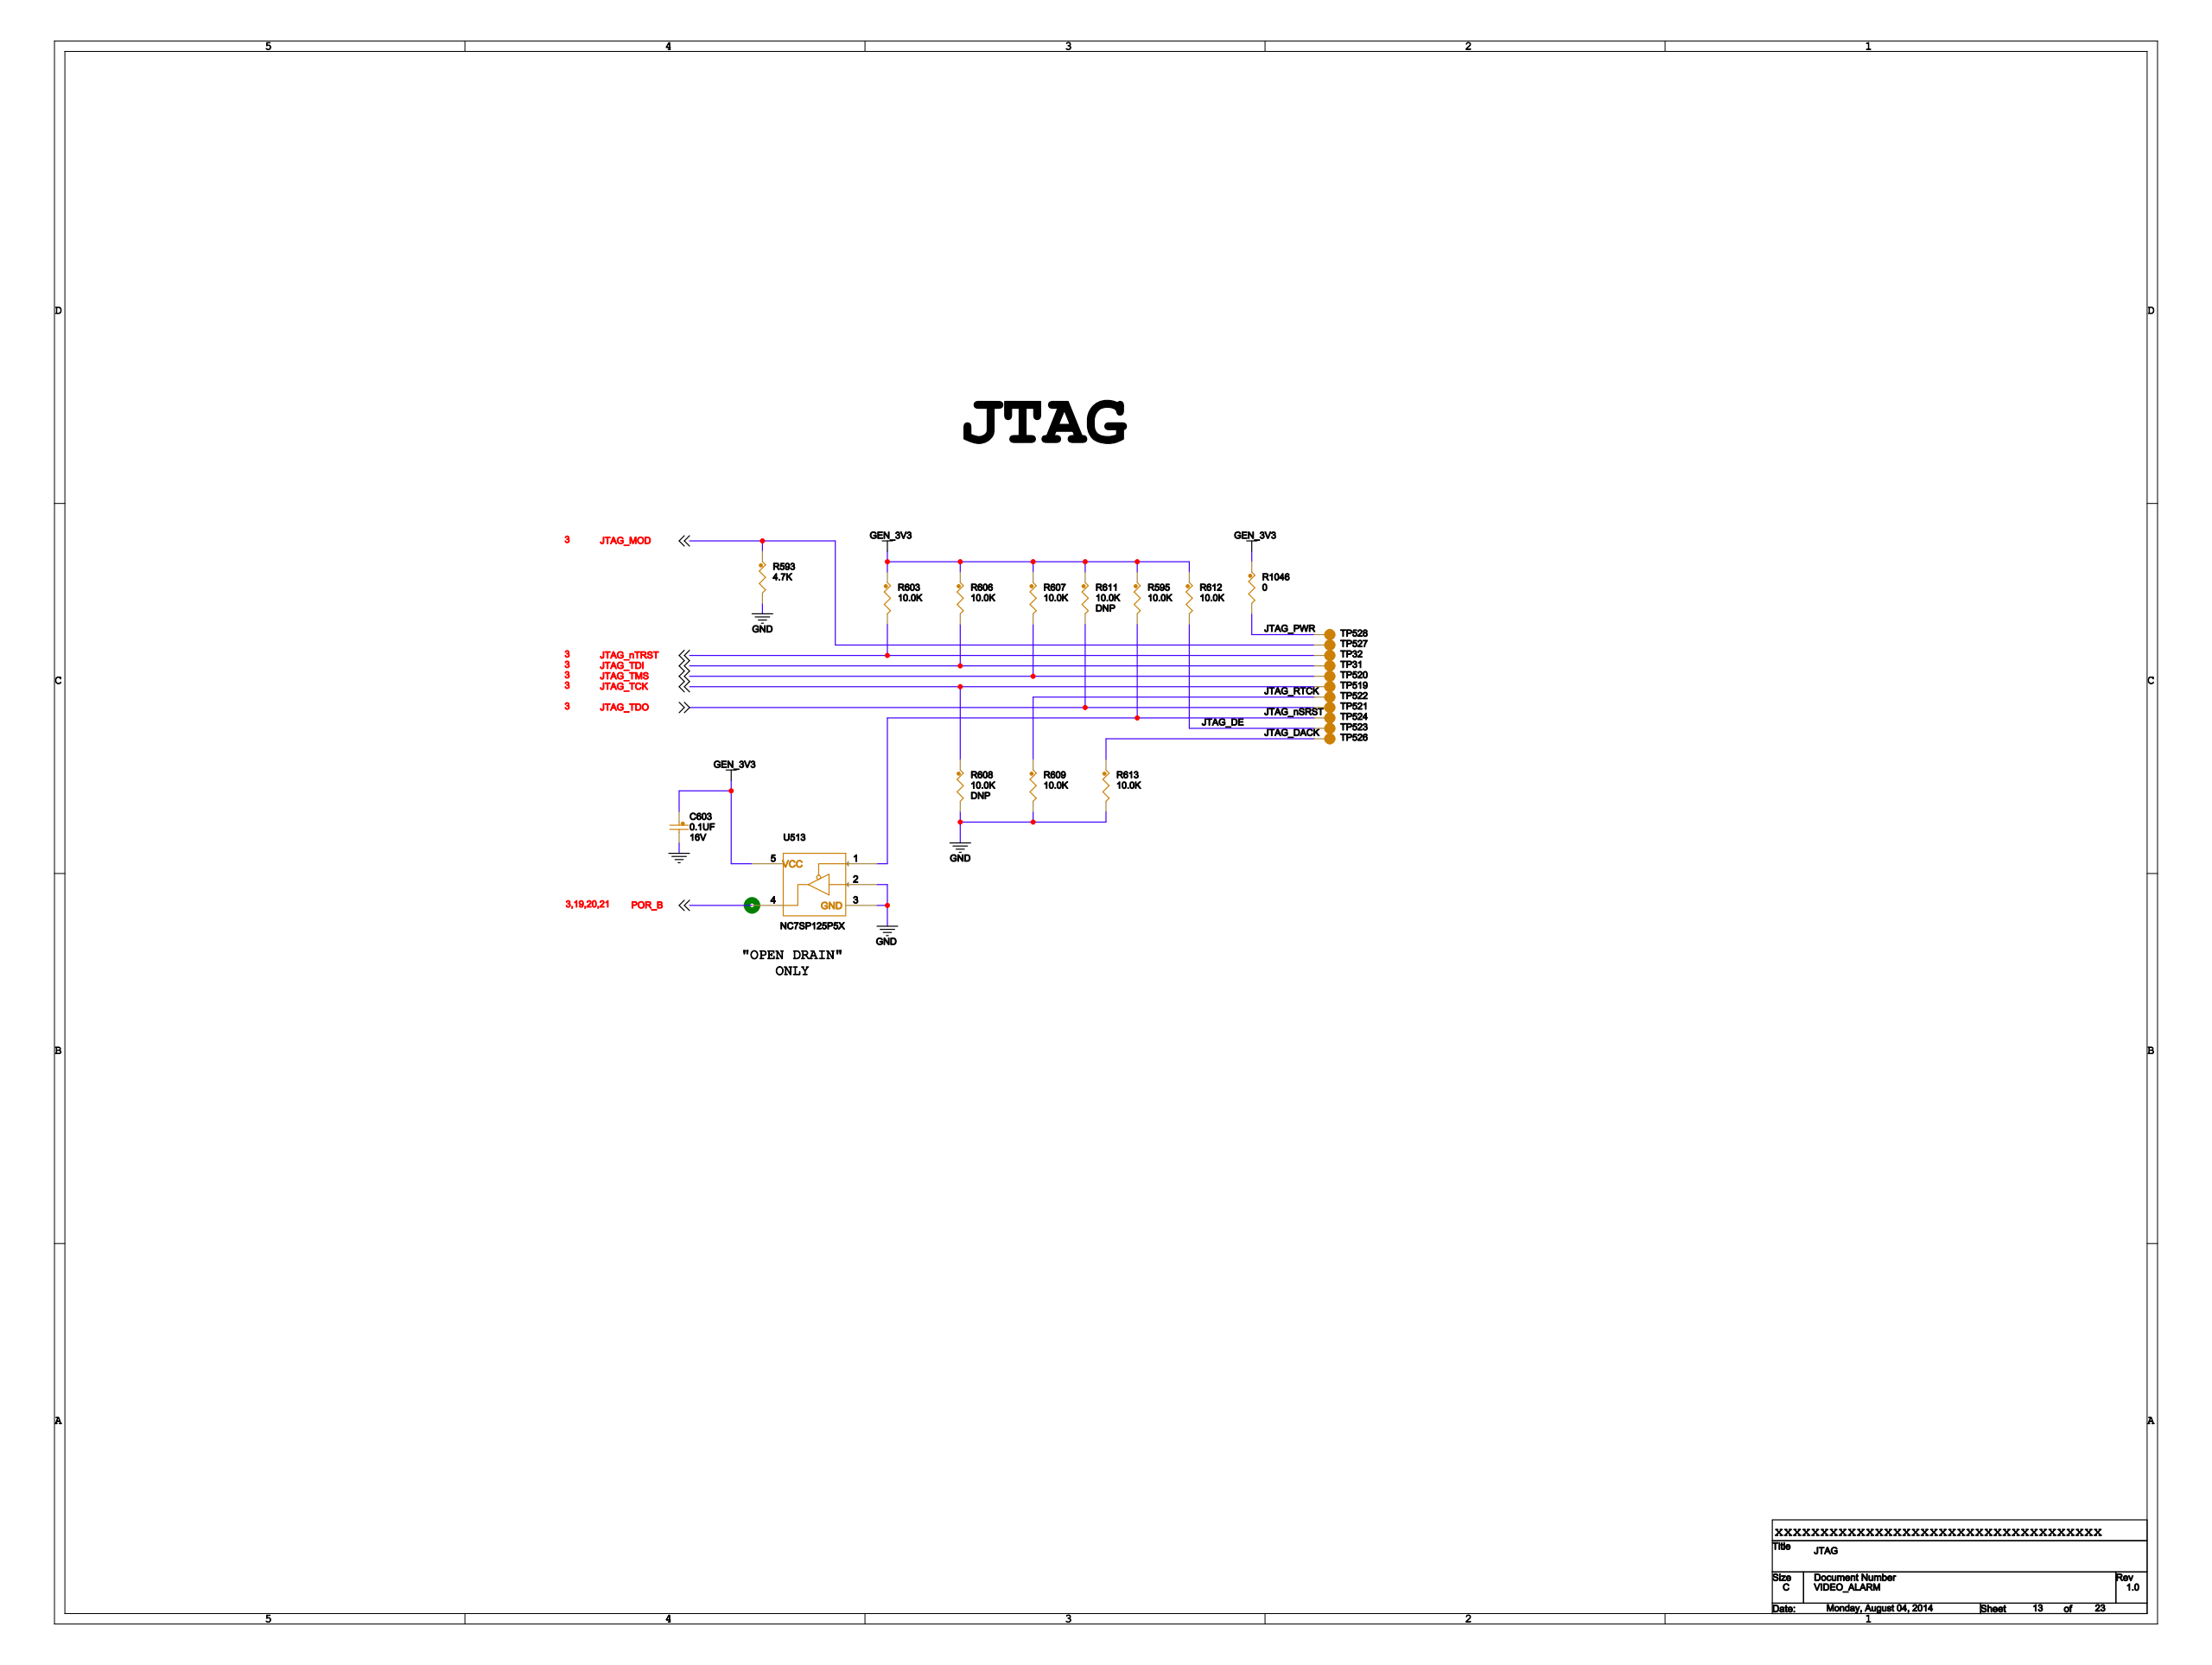Circuit board | Cadence Allegro | 994 parts | 728 nets | one sheet of the schematic
Parts on this sheet (reference | value | footprint):
C603 | 0.1UF | 0603_CC
R593 | 4.7K | 0603_CC
R595 | 10.0K | 0603_CC
R603 | 10.0K | 0603_CC
R606 | 10.0K | 0603_CC
R607 | 10.0K | 0603_CC
R608 | 10.0K | 0603_CC
R609 | 10.0K | 0603_CC
R611 | 10.0K | 0603_CC
R612 | 10.0K | 0603_CC
R613 | 10.0K | 0603_CC
R1046 | 0 | 0603_CC
TP31 | TPAD_020 | TPAD_020
TP32 | TPAD_020 | TPAD_020
TP519 | TPAD_020 | TPAD_020
TP520 | TPAD_020 | TPAD_020
TP521 | TPAD_020 | TPAD_020
TP522 | TPAD_020 | TPAD_020
TP523 | TPAD_020 | TPAD_020
TP524 | TPAD_020 | TPAD_020
TP526 | TPAD_020 | TPAD_020
TP527 | TPAD_020 | TPAD_020
TP528 | TPAD_020 | TPAD_020
U513 | NC7SP125P5X | SC70-5_A
Nets of these parts (net: part-pin ...):
GND: C603-2 R593-2 R608-2 R609-2 R613-2 U513-2 U513-3
POR_B: U513-4
GEN_3V3: C603-1 R595-1 R603-1 R606-1 R607-1 R611-1 R612-1 R1046-1 U513-5
JTAG_PWR: R1046-2 TP528-1
JTAG_DACK: R613-1 TP526-1
JTAG_DE: R612-2 TP523-1
JTAG_TDO: R611-2 TP521-1
JTAG_RTCK: R609-1 TP522-1
JTAG_TCK: R608-1 TP519-1
JTAG_TMS: R607-2 TP520-1
JTAG_TDI: R606-2 TP31-1
JTAG_NTRST: R603-2 TP32-1
JTAG_NSRST: R595-2 TP524-1 U513-1
JTAG_MOD: R593-1 TP527-1